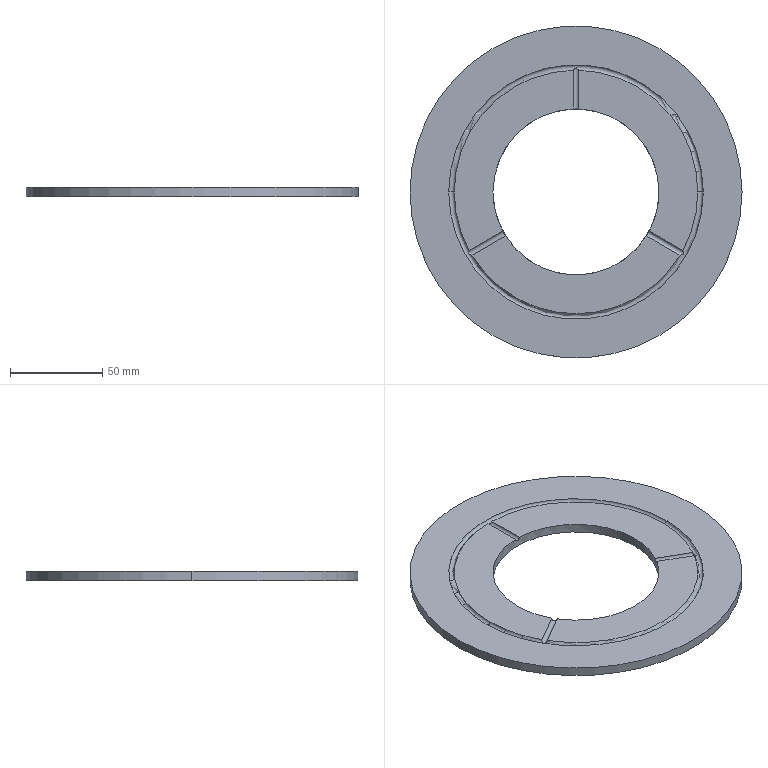Part | SolidWorks | features CirPattern 1, Extrusion 1, ICE 1, SweepCut 1 | 1 solid | 15 faces | box 180 x 180 x 5 mm | volume 93702 mm3 | cylinder 8 | plane 5 | torus 2 | commonest cylinder face diameters 3 x4 90 x2 180 x2
STEP:
#1=CARTESIAN_POINT('',(0.,67.5,3.5));
#2=VERTEX_POINT('',#1);
#3=CARTESIAN_POINT('',(1.5,65.983,5.));
#4=VERTEX_POINT('',#3);
#5=CARTESIAN_POINT('',(0.,67.5,3.5));
#6=CARTESIAN_POINT('',(0.0839,67.416,3.5));
#7=CARTESIAN_POINT('',(0.1692,67.331,3.507));
#8=CARTESIAN_POINT('',(0.3357,67.163,3.536));
#9=CARTESIAN_POINT('',(0.4181,67.081,3.557));
#10=CARTESIAN_POINT('',(0.6621,66.835,3.643));
#11=CARTESIAN_POINT('',(0.8218,66.673,3.731));
#12=CARTESIAN_POINT('',(1.11,66.381,3.974));
#13=CARTESIAN_POINT('',(1.242,66.246,4.131));
#14=CARTESIAN_POINT('',(1.39,66.096,4.425));
#15=CARTESIAN_POINT('',(1.43,66.055,4.531));
#16=CARTESIAN_POINT('',(1.485,65.998,4.758));
#17=CARTESIAN_POINT('',(1.5,65.983,4.879));
#18=CARTESIAN_POINT('',(1.5,65.983,5.));
#19=B_SPLINE_CURVE_WITH_KNOTS('',3,(#5,#6,#7,#8,#9,#10,#11,#12,#13,#14,#15,#16,#17,#18),.UNSPECIFIED.,.F.,.F.,(4,2,2,2,2,2,4),(-0.000007746,0.0003482,0.0007042,0.001416,0.002128,0.002484,0.00284),.UNSPECIFIED.);
#20=EDGE_CURVE('',#2,#4,#19,.T.);
#21=ORIENTED_EDGE('',*,*,#20,.F.);
#22=CARTESIAN_POINT('',(0.,45.,3.5));
#23=VERTEX_POINT('',#22);
#24=CARTESIAN_POINT('',(0.,67.5,3.5));
#25=DIRECTION('',(0.,-1.,0.));
#26=VECTOR('',#25,1000.);
#27=LINE('',#24,#26);
#28=EDGE_CURVE('',#2,#23,#27,.T.);
#29=ORIENTED_EDGE('',*,*,#28,.T.);
#30=CARTESIAN_POINT('',(1.5,44.975,5.));
#31=VERTEX_POINT('',#30);
#32=CARTESIAN_POINT('',(1.5,44.975,5.));
#33=CARTESIAN_POINT('',(1.5,44.975,4.901));
#34=CARTESIAN_POINT('',(1.49,44.975,4.803));
#35=CARTESIAN_POINT('',(1.452,44.977,4.612));
#36=CARTESIAN_POINT('',(1.423,44.978,4.516));
#37=CARTESIAN_POINT('',(1.348,44.98,4.335));
#38=CARTESIAN_POINT('',(1.302,44.981,4.248));
#39=CARTESIAN_POINT('',(1.193,44.984,4.085));
#40=CARTESIAN_POINT('',(1.13,44.986,4.008));
#41=CARTESIAN_POINT('',(0.9218,44.991,3.801));
#42=CARTESIAN_POINT('',(0.7544,44.994,3.689));
#43=CARTESIAN_POINT('',(0.3932,44.999,3.539));
#44=CARTESIAN_POINT('',(0.1957,45.,3.5));
#45=CARTESIAN_POINT('',(0.,45.,3.5));
#46=B_SPLINE_CURVE_WITH_KNOTS('',3,(#32,#33,#34,#35,#36,#37,#38,#39,#40,#41,#42,#43,#44,#45),.UNSPECIFIED.,.F.,.F.,(4,2,2,2,2,2,4),(0.,0.0002932,0.0005864,0.0008796,0.001173,0.001759,0.002346),.UNSPECIFIED.);
#47=EDGE_CURVE('',#31,#23,#46,.T.);
#48=ORIENTED_EDGE('',*,*,#47,.F.);
#49=CARTESIAN_POINT('',(1.5,67.5,5.));
#50=DIRECTION('',(0.,-1.,0.));
#51=VECTOR('',#50,1000.);
#52=LINE('',#49,#51);
#53=EDGE_CURVE('',#4,#31,#52,.T.);
#54=ORIENTED_EDGE('',*,*,#53,.F.);
#55=EDGE_LOOP('',(#21,#29,#48,#54));
#56=FACE_OUTER_BOUND('',#55,.T.);
#57=CARTESIAN_POINT('',(0.,67.5,5.));
#58=DIRECTION('',(0.,-1.,0.));
#59=DIRECTION('',(0.,0.,-1.));
#60=AXIS2_PLACEMENT_3D('',#57,#58,#59);
#61=CYLINDRICAL_SURFACE('',#60,1.5);
#62=ADVANCED_FACE('',(#56),#61,.F.);
#63=CARTESIAN_POINT('',(90.,0.,5.));
#64=VERTEX_POINT('',#63);
#65=CARTESIAN_POINT('',(-90.,0.,5.));
#66=VERTEX_POINT('',#65);
#67=CARTESIAN_POINT('',(0.,0.,5.));
#68=DIRECTION('',(0.,0.,1.));
#69=DIRECTION('',(1.,0.,0.));
#70=AXIS2_PLACEMENT_3D('',#67,#68,#69);
#71=CIRCLE('',#70,90.);
#72=EDGE_CURVE('',#64,#66,#71,.T.);
#73=ORIENTED_EDGE('',*,*,#72,.F.);
#74=CARTESIAN_POINT('',(90.,0.,0.));
#75=VERTEX_POINT('',#74);
#76=CARTESIAN_POINT('',(90.,0.,5.));
#77=DIRECTION('',(0.,0.,-1.));
#78=VECTOR('',#77,1000.);
#79=LINE('',#76,#78);
#80=EDGE_CURVE('',#64,#75,#79,.T.);
#81=ORIENTED_EDGE('',*,*,#80,.T.);
#82=CARTESIAN_POINT('',(-90.,0.,0.));
#83=VERTEX_POINT('',#82);
#84=CARTESIAN_POINT('',(0.,0.,0.));
#85=DIRECTION('',(0.,0.,1.));
#86=DIRECTION('',(1.,0.,0.));
#87=AXIS2_PLACEMENT_3D('',#84,#85,#86);
#88=CIRCLE('',#87,90.);
#89=EDGE_CURVE('',#75,#83,#88,.T.);
#90=ORIENTED_EDGE('',*,*,#89,.T.);
#91=CARTESIAN_POINT('',(-90.,0.,5.));
#92=DIRECTION('',(0.,0.,-1.));
#93=VECTOR('',#92,1000.);
#94=LINE('',#91,#93);
#95=EDGE_CURVE('',#66,#83,#94,.T.);
#96=ORIENTED_EDGE('',*,*,#95,.F.);
#97=EDGE_LOOP('',(#73,#81,#90,#96));
#98=FACE_OUTER_BOUND('',#97,.T.);
#99=CARTESIAN_POINT('',(0.,0.,5.));
#100=DIRECTION('',(0.,0.,-1.));
#101=DIRECTION('',(-1.,0.,0.));
#102=AXIS2_PLACEMENT_3D('',#99,#100,#101);
#103=CYLINDRICAL_SURFACE('',#102,90.);
#104=ADVANCED_FACE('',(#98),#103,.T.);
#105=CARTESIAN_POINT('',(-66.,0.,5.));
#106=VERTEX_POINT('',#105);
#107=CARTESIAN_POINT('',(-57.893,-31.692,5.));
#108=VERTEX_POINT('',#107);
#109=CARTESIAN_POINT('',(0.,0.,5.));
#110=DIRECTION('',(0.,0.,1.));
#111=DIRECTION('',(-1.,0.,0.));
#112=AXIS2_PLACEMENT_3D('',#109,#110,#111);
#113=CIRCLE('',#112,66.);
#114=EDGE_CURVE('',#106,#108,#113,.T.);
#115=ORIENTED_EDGE('',*,*,#114,.F.);
#116=CARTESIAN_POINT('',(-69.,0.,5.));
#117=VERTEX_POINT('',#116);
#118=CARTESIAN_POINT('',(-67.5,0.,5.));
#119=DIRECTION('',(0.,1.,0.));
#120=DIRECTION('',(-1.,0.,0.));
#121=AXIS2_PLACEMENT_3D('',#118,#119,#120);
#122=CIRCLE('',#121,1.5);
#123=EDGE_CURVE('',#106,#117,#122,.T.);
#124=ORIENTED_EDGE('',*,*,#123,.T.);
#125=CARTESIAN_POINT('',(69.,0.,5.));
#126=VERTEX_POINT('',#125);
#127=CARTESIAN_POINT('',(0.,0.,5.));
#128=DIRECTION('',(0.,0.,-1.));
#129=DIRECTION('',(1.,0.,0.));
#130=AXIS2_PLACEMENT_3D('',#127,#128,#129);
#131=CIRCLE('',#130,69.);
#132=EDGE_CURVE('',#126,#117,#131,.T.);
#133=ORIENTED_EDGE('',*,*,#132,.F.);
#134=CARTESIAN_POINT('',(66.,0.,5.));
#135=VERTEX_POINT('',#134);
#136=CARTESIAN_POINT('',(67.5,0.,5.));
#137=DIRECTION('',(0.,-1.,0.));
#138=DIRECTION('',(0.,0.,-1.));
#139=AXIS2_PLACEMENT_3D('',#136,#137,#138);
#140=CIRCLE('',#139,1.5);
#141=EDGE_CURVE('',#135,#126,#140,.T.);
#142=ORIENTED_EDGE('',*,*,#141,.F.);
#143=CARTESIAN_POINT('',(57.893,-31.692,5.));
#144=VERTEX_POINT('',#143);
#145=CARTESIAN_POINT('',(0.,0.,5.));
#146=DIRECTION('',(0.,0.,1.));
#147=DIRECTION('',(-1.,0.,0.));
#148=AXIS2_PLACEMENT_3D('',#145,#146,#147);
#149=CIRCLE('',#148,66.);
#150=EDGE_CURVE('',#144,#135,#149,.T.);
#151=ORIENTED_EDGE('',*,*,#150,.F.);
#152=CARTESIAN_POINT('',(58.457,-33.75,3.5));
#153=VERTEX_POINT('',#152);
#154=CARTESIAN_POINT('',(57.893,-31.692,5.));
#155=CARTESIAN_POINT('',(57.893,-31.692,4.757));
#156=CARTESIAN_POINT('',(57.916,-31.776,4.524));
#157=CARTESIAN_POINT('',(57.992,-32.046,4.133));
#158=CARTESIAN_POINT('',(58.042,-32.226,3.976));
#159=CARTESIAN_POINT('',(58.151,-32.624,3.731));
#160=CARTESIAN_POINT('',(58.21,-32.838,3.645));
#161=CARTESIAN_POINT('',(58.333,-33.289,3.528));
#162=CARTESIAN_POINT('',(58.395,-33.52,3.5));
#163=CARTESIAN_POINT('',(58.457,-33.75,3.5));
#164=B_SPLINE_CURVE_WITH_KNOTS('',3,(#154,#155,#156,#157,#158,#159,#160,#161,#162,#163),.UNSPECIFIED.,.F.,.F.,(4,2,2,2,4),(0.000000196,0.000716,0.001432,0.002147,0.002863),.UNSPECIFIED.);
#165=EDGE_CURVE('',#144,#153,#164,.T.);
#166=ORIENTED_EDGE('',*,*,#165,.T.);
#167=CARTESIAN_POINT('',(56.393,-34.291,5.));
#168=VERTEX_POINT('',#167);
#169=CARTESIAN_POINT('',(58.457,-33.75,3.5));
#170=CARTESIAN_POINT('',(58.342,-33.781,3.5));
#171=CARTESIAN_POINT('',(58.225,-33.812,3.507));
#172=CARTESIAN_POINT('',(57.997,-33.872,3.536));
#173=CARTESIAN_POINT('',(57.885,-33.902,3.557));
#174=CARTESIAN_POINT('',(57.55,-33.991,3.643));
#175=CARTESIAN_POINT('',(57.33,-34.048,3.731));
#176=CARTESIAN_POINT('',(56.932,-34.152,3.974));
#177=CARTESIAN_POINT('',(56.75,-34.199,4.131));
#178=CARTESIAN_POINT('',(56.546,-34.251,4.425));
#179=CARTESIAN_POINT('',(56.49,-34.266,4.531));
#180=CARTESIAN_POINT('',(56.414,-34.285,4.758));
#181=CARTESIAN_POINT('',(56.393,-34.291,4.879));
#182=CARTESIAN_POINT('',(56.393,-34.291,5.));
#183=B_SPLINE_CURVE_WITH_KNOTS('',3,(#169,#170,#171,#172,#173,#174,#175,#176,#177,#178,#179,#180,#181,#182),.UNSPECIFIED.,.F.,.F.,(4,2,2,2,2,2,4),(-0.000007746,0.0003482,0.0007042,0.001416,0.002128,0.002484,0.00284),.UNSPECIFIED.);
#184=EDGE_CURVE('',#153,#168,#183,.T.);
#185=ORIENTED_EDGE('',*,*,#184,.T.);
#186=CARTESIAN_POINT('',(-56.393,-34.291,5.));
#187=VERTEX_POINT('',#186);
#188=CARTESIAN_POINT('',(0.,0.,5.));
#189=DIRECTION('',(0.,0.,1.));
#190=DIRECTION('',(-1.,0.,0.));
#191=AXIS2_PLACEMENT_3D('',#188,#189,#190);
#192=CIRCLE('',#191,66.);
#193=EDGE_CURVE('',#187,#168,#192,.T.);
#194=ORIENTED_EDGE('',*,*,#193,.F.);
#195=CARTESIAN_POINT('',(-58.457,-33.75,3.5));
#196=VERTEX_POINT('',#195);
#197=CARTESIAN_POINT('',(-56.393,-34.291,5.));
#198=CARTESIAN_POINT('',(-56.393,-34.291,4.757));
#199=CARTESIAN_POINT('',(-56.477,-34.269,4.524));
#200=CARTESIAN_POINT('',(-56.748,-34.199,4.133));
#201=CARTESIAN_POINT('',(-56.929,-34.153,3.976));
#202=CARTESIAN_POINT('',(-57.329,-34.049,3.731));
#203=CARTESIAN_POINT('',(-57.544,-33.992,3.645));
#204=CARTESIAN_POINT('',(-57.995,-33.873,3.528));
#205=CARTESIAN_POINT('',(-58.226,-33.812,3.5));
#206=CARTESIAN_POINT('',(-58.457,-33.75,3.5));
#207=B_SPLINE_CURVE_WITH_KNOTS('',3,(#197,#198,#199,#200,#201,#202,#203,#204,#205,#206),.UNSPECIFIED.,.F.,.F.,(4,2,2,2,4),(0.000000196,0.000716,0.001432,0.002147,0.002863),.UNSPECIFIED.);
#208=EDGE_CURVE('',#187,#196,#207,.T.);
#209=ORIENTED_EDGE('',*,*,#208,.T.);
#210=CARTESIAN_POINT('',(-58.457,-33.75,3.5));
#211=CARTESIAN_POINT('',(-58.426,-33.635,3.5));
#212=CARTESIAN_POINT('',(-58.395,-33.519,3.507));
#213=CARTESIAN_POINT('',(-58.333,-33.291,3.536));
#214=CARTESIAN_POINT('',(-58.303,-33.178,3.557));
#215=CARTESIAN_POINT('',(-58.212,-32.844,3.643));
#216=CARTESIAN_POINT('',(-58.152,-32.625,3.731));
#217=CARTESIAN_POINT('',(-58.042,-32.229,3.974));
#218=CARTESIAN_POINT('',(-57.992,-32.048,4.131));
#219=CARTESIAN_POINT('',(-57.935,-31.844,4.425));
#220=CARTESIAN_POINT('',(-57.92,-31.789,4.531));
#221=CARTESIAN_POINT('',(-57.899,-31.713,4.758));
#222=CARTESIAN_POINT('',(-57.893,-31.692,4.879));
#223=CARTESIAN_POINT('',(-57.893,-31.692,5.));
#224=B_SPLINE_CURVE_WITH_KNOTS('',3,(#210,#211,#212,#213,#214,#215,#216,#217,#218,#219,#220,#221,#222,#223),.UNSPECIFIED.,.F.,.F.,(4,2,2,2,2,2,4),(-0.000007746,0.0003482,0.0007042,0.001416,0.002128,0.002484,0.00284),.UNSPECIFIED.);
#225=EDGE_CURVE('',#196,#108,#224,.T.);
#226=ORIENTED_EDGE('',*,*,#225,.T.);
#227=EDGE_LOOP('',(#115,#124,#133,#142,#151,#166,#185,#194,#209,#226));
#228=FACE_OUTER_BOUND('',#227,.T.);
#229=CARTESIAN_POINT('',(0.,0.,5.));
#230=DIRECTION('',(0.,0.,1.));
#231=DIRECTION('',(1.,0.,0.));
#232=AXIS2_PLACEMENT_3D('',#229,#230,#231);
#233=TOROIDAL_SURFACE('',#232,67.5,1.5);
#234=ADVANCED_FACE('',(#228),#233,.F.);
#235=CARTESIAN_POINT('',(39.699,-21.188,5.));
#236=VERTEX_POINT('',#235);
#237=CARTESIAN_POINT('',(45.,0.,5.));
#238=VERTEX_POINT('',#237);
#239=CARTESIAN_POINT('',(0.,0.,5.));
#240=DIRECTION('',(0.,0.,1.));
#241=DIRECTION('',(1.,0.,0.));
#242=AXIS2_PLACEMENT_3D('',#239,#240,#241);
#243=CIRCLE('',#242,45.);
#244=EDGE_CURVE('',#236,#238,#243,.T.);
#245=ORIENTED_EDGE('',*,*,#244,.T.);
#246=CARTESIAN_POINT('',(45.,0.,0.));
#247=VERTEX_POINT('',#246);
#248=CARTESIAN_POINT('',(45.,0.,5.));
#249=DIRECTION('',(0.,0.,-1.));
#250=VECTOR('',#249,1000.);
#251=LINE('',#248,#250);
#252=EDGE_CURVE('',#238,#247,#251,.T.);
#253=ORIENTED_EDGE('',*,*,#252,.T.);
#254=CARTESIAN_POINT('',(-45.,0.,0.));
#255=VERTEX_POINT('',#254);
#256=CARTESIAN_POINT('',(0.,0.,0.));
#257=DIRECTION('',(0.,0.,1.));
#258=DIRECTION('',(1.,0.,0.));
#259=AXIS2_PLACEMENT_3D('',#256,#257,#258);
#260=CIRCLE('',#259,45.);
#261=EDGE_CURVE('',#255,#247,#260,.T.);
#262=ORIENTED_EDGE('',*,*,#261,.F.);
#263=CARTESIAN_POINT('',(-45.,0.,5.));
#264=VERTEX_POINT('',#263);
#265=CARTESIAN_POINT('',(-45.,0.,5.));
#266=DIRECTION('',(0.,0.,-1.));
#267=VECTOR('',#266,1000.);
#268=LINE('',#265,#267);
#269=EDGE_CURVE('',#264,#255,#268,.T.);
#270=ORIENTED_EDGE('',*,*,#269,.F.);
#271=CARTESIAN_POINT('',(-39.699,-21.188,5.));
#272=VERTEX_POINT('',#271);
#273=CARTESIAN_POINT('',(0.,0.,5.));
#274=DIRECTION('',(0.,0.,1.));
#275=DIRECTION('',(1.,0.,0.));
#276=AXIS2_PLACEMENT_3D('',#273,#274,#275);
#277=CIRCLE('',#276,45.);
#278=EDGE_CURVE('',#264,#272,#277,.T.);
#279=ORIENTED_EDGE('',*,*,#278,.T.);
#280=CARTESIAN_POINT('',(-38.199,-23.787,5.));
#281=VERTEX_POINT('',#280);
#282=CARTESIAN_POINT('',(-39.699,-21.188,5.));
#283=CARTESIAN_POINT('',(-39.699,-21.188,4.901));
#284=CARTESIAN_POINT('',(-39.695,-21.197,4.803));
#285=CARTESIAN_POINT('',(-39.677,-21.231,4.612));
#286=CARTESIAN_POINT('',(-39.663,-21.256,4.516));
#287=CARTESIAN_POINT('',(-39.628,-21.323,4.335));
#288=CARTESIAN_POINT('',(-39.606,-21.363,4.249));
#289=CARTESIAN_POINT('',(-39.554,-21.459,4.086));
#290=CARTESIAN_POINT('',(-39.524,-21.515,4.008));
#291=CARTESIAN_POINT('',(-39.424,-21.697,3.801));
#292=CARTESIAN_POINT('',(-39.343,-21.843,3.689));
#293=CARTESIAN_POINT('',(-39.167,-22.158,3.539));
#294=CARTESIAN_POINT('',(-39.069,-22.33,3.5));
#295=CARTESIAN_POINT('',(-38.922,-22.584,3.5));
#296=CARTESIAN_POINT('',(-38.873,-22.67,3.51));
#297=CARTESIAN_POINT('',(-38.775,-22.836,3.548));
#298=CARTESIAN_POINT('',(-38.728,-22.917,3.576));
#299=CARTESIAN_POINT('',(-38.635,-23.073,3.651));
#300=CARTESIAN_POINT('',(-38.59,-23.148,3.698));
#301=CARTESIAN_POINT('',(-38.506,-23.287,3.807));
#302=CARTESIAN_POINT('',(-38.467,-23.352,3.869));
#303=CARTESIAN_POINT('',(-38.357,-23.532,4.079));
#304=CARTESIAN_POINT('',(-38.299,-23.625,4.244));
#305=CARTESIAN_POINT('',(-38.24,-23.722,4.517));
#306=CARTESIAN_POINT('',(-38.225,-23.746,4.61));
#307=CARTESIAN_POINT('',(-38.205,-23.778,4.803));
#308=CARTESIAN_POINT('',(-38.199,-23.787,4.902));
#309=CARTESIAN_POINT('',(-38.199,-23.787,5.));
#310=B_SPLINE_CURVE_WITH_KNOTS('',3,(#282,#283,#284,#285,#286,#287,#288,#289,#290,#291,#292,#293,#294,#295,#296,#297,#298,#299,#300,#301,#302,#303,#304,#305,#306,#307,#308,#309),.UNSPECIFIED.,.F.,.F.,(4,2,2,2,2,2,2,2,2,2,2,2,2,4),(0.,0.0002931,0.0005863,0.0008794,0.001173,0.001759,0.002345,0.002638,0.002931,0.003224,0.003518,0.004104,0.004397,0.00469),.UNSPECIFIED.);
#311=EDGE_CURVE('',#272,#281,#310,.T.);
#312=ORIENTED_EDGE('',*,*,#311,.T.);
#313=CARTESIAN_POINT('',(38.199,-23.787,5.));
#314=VERTEX_POINT('',#313);
#315=CARTESIAN_POINT('',(0.,0.,5.));
#316=DIRECTION('',(0.,0.,1.));
#317=DIRECTION('',(1.,0.,0.));
#318=AXIS2_PLACEMENT_3D('',#315,#316,#317);
#319=CIRCLE('',#318,45.);
#320=EDGE_CURVE('',#281,#314,#319,.T.);
#321=ORIENTED_EDGE('',*,*,#320,.T.);
#322=CARTESIAN_POINT('',(38.199,-23.787,5.));
#323=CARTESIAN_POINT('',(38.199,-23.787,4.901));
#324=CARTESIAN_POINT('',(38.205,-23.778,4.803));
#325=CARTESIAN_POINT('',(38.225,-23.746,4.612));
#326=CARTESIAN_POINT('',(38.24,-23.721,4.516));
#327=CARTESIAN_POINT('',(38.28,-23.657,4.335));
#328=CARTESIAN_POINT('',(38.304,-23.618,4.249));
#329=CARTESIAN_POINT('',(38.361,-23.525,4.086));
#330=CARTESIAN_POINT('',(38.394,-23.471,4.008));
#331=CARTESIAN_POINT('',(38.502,-23.294,3.801));
#332=CARTESIAN_POINT('',(38.589,-23.151,3.689));
#333=CARTESIAN_POINT('',(38.773,-22.84,3.539));
#334=CARTESIAN_POINT('',(38.873,-22.67,3.5));
#335=CARTESIAN_POINT('',(39.02,-22.416,3.5));
#336=CARTESIAN_POINT('',(39.069,-22.329,3.51));
#337=CARTESIAN_POINT('',(39.164,-22.162,3.548));
#338=CARTESIAN_POINT('',(39.21,-22.081,3.576));
#339=CARTESIAN_POINT('',(39.299,-21.922,3.651));
#340=CARTESIAN_POINT('',(39.342,-21.846,3.698));
#341=CARTESIAN_POINT('',(39.42,-21.703,3.807));
#342=CARTESIAN_POINT('',(39.457,-21.637,3.869));
#343=CARTESIAN_POINT('',(39.558,-21.452,4.079));
#344=CARTESIAN_POINT('',(39.61,-21.356,4.244));
#345=CARTESIAN_POINT('',(39.663,-21.256,4.517));
#346=CARTESIAN_POINT('',(39.677,-21.231,4.61));
#347=CARTESIAN_POINT('',(39.695,-21.197,4.803));
#348=CARTESIAN_POINT('',(39.699,-21.188,4.902));
#349=CARTESIAN_POINT('',(39.699,-21.188,5.));
#350=B_SPLINE_CURVE_WITH_KNOTS('',3,(#322,#323,#324,#325,#326,#327,#328,#329,#330,#331,#332,#333,#334,#335,#336,#337,#338,#339,#340,#341,#342,#343,#344,#345,#346,#347,#348,#349),.UNSPECIFIED.,.F.,.F.,(4,2,2,2,2,2,2,2,2,2,2,2,2,4),(0.,0.0002931,0.0005863,0.0008794,0.001173,0.001759,0.002345,0.002638,0.002931,0.003224,0.003518,0.004104,0.004397,0.00469),.UNSPECIFIED.);
#351=EDGE_CURVE('',#314,#236,#350,.T.);
#352=ORIENTED_EDGE('',*,*,#351,.T.);
#353=EDGE_LOOP('',(#245,#253,#262,#270,#279,#312,#321,#352));
#354=FACE_OUTER_BOUND('',#353,.T.);
#355=CARTESIAN_POINT('',(0.,0.,5.));
#356=DIRECTION('',(0.,0.,-1.));
#357=DIRECTION('',(-1.,0.,0.));
#358=AXIS2_PLACEMENT_3D('',#355,#356,#357);
#359=CYLINDRICAL_SURFACE('',#358,45.);
#360=ADVANCED_FACE('',(#354),#359,.F.);
#361=ORIENTED_EDGE('',*,*,#244,.F.);
#362=CARTESIAN_POINT('',(59.207,-32.451,5.));
#363=DIRECTION('',(0.866,-0.5,0.));
#364=VECTOR('',#363,1000.);
#365=LINE('',#362,#364);
#366=EDGE_CURVE('',#236,#144,#365,.T.);
#367=ORIENTED_EDGE('',*,*,#366,.T.);
#368=ORIENTED_EDGE('',*,*,#150,.T.);
#369=CARTESIAN_POINT('',(0.,0.,5.));
#370=DIRECTION('',(0.,0.,1.));
#371=DIRECTION('',(-1.,0.,0.));
#372=AXIS2_PLACEMENT_3D('',#369,#370,#371);
#373=CIRCLE('',#372,66.);
#374=EDGE_CURVE('',#135,#4,#373,.T.);
#375=ORIENTED_EDGE('',*,*,#374,.T.);
#376=ORIENTED_EDGE('',*,*,#53,.T.);
#377=CARTESIAN_POINT('',(0.,0.,5.));
#378=DIRECTION('',(0.,0.,1.));
#379=DIRECTION('',(1.,0.,0.));
#380=AXIS2_PLACEMENT_3D('',#377,#378,#379);
#381=CIRCLE('',#380,45.);
#382=EDGE_CURVE('',#238,#31,#381,.T.);
#383=ORIENTED_EDGE('',*,*,#382,.F.);
#384=EDGE_LOOP('',(#361,#367,#368,#375,#376,#383));
#385=FACE_OUTER_BOUND('',#384,.T.);
#386=CARTESIAN_POINT('',(0.,0.,5.));
#387=DIRECTION('',(0.,0.,1.));
#388=DIRECTION('',(1.,0.,0.));
#389=AXIS2_PLACEMENT_3D('',#386,#387,#388);
#390=PLANE('',#389);
#391=ADVANCED_FACE('',(#385),#390,.T.);
#392=ORIENTED_EDGE('',*,*,#193,.T.);
#393=CARTESIAN_POINT('',(57.707,-35.049,5.));
#394=DIRECTION('',(-0.866,0.5,0.));
#395=VECTOR('',#394,1000.);
#396=LINE('',#393,#395);
#397=EDGE_CURVE('',#168,#314,#396,.T.);
#398=ORIENTED_EDGE('',*,*,#397,.T.);
#399=ORIENTED_EDGE('',*,*,#320,.F.);
#400=CARTESIAN_POINT('',(-57.707,-35.049,5.));
#401=DIRECTION('',(-0.866,-0.5,0.));
#402=VECTOR('',#401,1000.);
#403=LINE('',#400,#402);
#404=EDGE_CURVE('',#281,#187,#403,.T.);
#405=ORIENTED_EDGE('',*,*,#404,.T.);
#406=EDGE_LOOP('',(#392,#398,#399,#405));
#407=FACE_OUTER_BOUND('',#406,.T.);
#408=CARTESIAN_POINT('',(0.,0.,5.));
#409=DIRECTION('',(0.,0.,1.));
#410=DIRECTION('',(1.,0.,0.));
#411=AXIS2_PLACEMENT_3D('',#408,#409,#410);
#412=PLANE('',#411);
#413=ADVANCED_FACE('',(#407),#412,.T.);
#414=CARTESIAN_POINT('',(-1.5,65.983,5.));
#415=VERTEX_POINT('',#414);
#416=CARTESIAN_POINT('',(0.,0.,5.));
#417=DIRECTION('',(0.,0.,1.));
#418=DIRECTION('',(-1.,0.,0.));
#419=AXIS2_PLACEMENT_3D('',#416,#417,#418);
#420=CIRCLE('',#419,66.);
#421=EDGE_CURVE('',#415,#106,#420,.T.);
#422=ORIENTED_EDGE('',*,*,#421,.T.);
#423=ORIENTED_EDGE('',*,*,#114,.T.);
#424=CARTESIAN_POINT('',(-59.207,-32.451,5.));
#425=DIRECTION('',(0.866,0.5,0.));
#426=VECTOR('',#425,1000.);
#427=LINE('',#424,#426);
#428=EDGE_CURVE('',#108,#272,#427,.T.);
#429=ORIENTED_EDGE('',*,*,#428,.T.);
#430=ORIENTED_EDGE('',*,*,#278,.F.);
#431=CARTESIAN_POINT('',(-1.5,44.975,5.));
#432=VERTEX_POINT('',#431);
#433=CARTESIAN_POINT('',(0.,0.,5.));
#434=DIRECTION('',(0.,0.,1.));
#435=DIRECTION('',(1.,0.,0.));
#436=AXIS2_PLACEMENT_3D('',#433,#434,#435);
#437=CIRCLE('',#436,45.);
#438=EDGE_CURVE('',#432,#264,#437,.T.);
#439=ORIENTED_EDGE('',*,*,#438,.F.);
#440=CARTESIAN_POINT('',(-1.5,67.5,5.));
#441=DIRECTION('',(0.,1.,0.));
#442=VECTOR('',#441,1000.);
#443=LINE('',#440,#442);
#444=EDGE_CURVE('',#432,#415,#443,.T.);
#445=ORIENTED_EDGE('',*,*,#444,.T.);
#446=EDGE_LOOP('',(#422,#423,#429,#430,#439,#445));
#447=FACE_OUTER_BOUND('',#446,.T.);
#448=CARTESIAN_POINT('',(0.,0.,5.));
#449=DIRECTION('',(0.,0.,1.));
#450=DIRECTION('',(1.,0.,0.));
#451=AXIS2_PLACEMENT_3D('',#448,#449,#450);
#452=PLANE('',#451);
#453=ADVANCED_FACE('',(#447),#452,.T.);
#454=ORIENTED_EDGE('',*,*,#252,.F.);
#455=ORIENTED_EDGE('',*,*,#382,.T.);
#456=ORIENTED_EDGE('',*,*,#47,.T.);
#457=CARTESIAN_POINT('',(0.,45.,3.5));
#458=CARTESIAN_POINT('',(-0.09778,45.,3.5));
#459=CARTESIAN_POINT('',(-0.1971,45.,3.51));
#460=CARTESIAN_POINT('',(-0.3894,44.998,3.548));
#461=CARTESIAN_POINT('',(-0.4828,44.998,3.576));
#462=CARTESIAN_POINT('',(-0.6643,44.995,3.652));
#463=CARTESIAN_POINT('',(-0.7521,44.994,3.698));
#464=CARTESIAN_POINT('',(-0.9145,44.991,3.807));
#465=CARTESIAN_POINT('',(-0.9903,44.989,3.869));
#466=CARTESIAN_POINT('',(-1.2,44.984,4.079));
#467=CARTESIAN_POINT('',(-1.31,44.981,4.244));
#468=CARTESIAN_POINT('',(-1.461,44.976,4.607));
#469=CARTESIAN_POINT('',(-1.5,44.975,4.802));
#470=CARTESIAN_POINT('',(-1.5,44.975,5.));
#471=B_SPLINE_CURVE_WITH_KNOTS('',3,(#457,#458,#459,#460,#461,#462,#463,#464,#465,#466,#467,#468,#469,#470),.UNSPECIFIED.,.F.,.F.,(4,2,2,2,2,2,4),(0.002346,0.002638,0.002931,0.003224,0.003517,0.004103,0.004689),.UNSPECIFIED.);
#472=EDGE_CURVE('',#23,#432,#471,.T.);
#473=ORIENTED_EDGE('',*,*,#472,.T.);
#474=ORIENTED_EDGE('',*,*,#438,.T.);
#475=ORIENTED_EDGE('',*,*,#269,.T.);
#476=CARTESIAN_POINT('',(0.,0.,0.));
#477=DIRECTION('',(0.,0.,1.));
#478=DIRECTION('',(1.,0.,0.));
#479=AXIS2_PLACEMENT_3D('',#476,#477,#478);
#480=CIRCLE('',#479,45.);
#481=EDGE_CURVE('',#247,#255,#480,.T.);
#482=ORIENTED_EDGE('',*,*,#481,.F.);
#483=EDGE_LOOP('',(#454,#455,#456,#473,#474,#475,#482));
#484=FACE_OUTER_BOUND('',#483,.T.);
#485=CARTESIAN_POINT('',(0.,0.,5.));
#486=DIRECTION('',(0.,0.,-1.));
#487=DIRECTION('',(-1.,0.,0.));
#488=AXIS2_PLACEMENT_3D('',#485,#486,#487);
#489=CYLINDRICAL_SURFACE('',#488,45.);
#490=ADVANCED_FACE('',(#484),#489,.F.);
#491=ORIENTED_EDGE('',*,*,#123,.F.);
#492=ORIENTED_EDGE('',*,*,#421,.F.);
#493=CARTESIAN_POINT('',(-1.5,65.983,5.));
#494=CARTESIAN_POINT('',(-1.5,65.983,4.757));
#495=CARTESIAN_POINT('',(-1.439,66.045,4.524));
#496=CARTESIAN_POINT('',(-1.243,66.245,4.133));
#497=CARTESIAN_POINT('',(-1.112,66.379,3.976));
#498=CARTESIAN_POINT('',(-0.8224,66.673,3.731));
#499=CARTESIAN_POINT('',(-0.6665,66.83,3.645));
#500=CARTESIAN_POINT('',(-0.3376,67.162,3.528));
#501=CARTESIAN_POINT('',(-0.1687,67.331,3.5));
#502=CARTESIAN_POINT('',(0.,67.5,3.5));
#503=B_SPLINE_CURVE_WITH_KNOTS('',3,(#493,#494,#495,#496,#497,#498,#499,#500,#501,#502),.UNSPECIFIED.,.F.,.F.,(4,2,2,2,4),(0.000000196,0.000716,0.001432,0.002147,0.002863),.UNSPECIFIED.);
#504=EDGE_CURVE('',#415,#2,#503,.T.);
#505=ORIENTED_EDGE('',*,*,#504,.T.);
#506=ORIENTED_EDGE('',*,*,#20,.T.);
#507=ORIENTED_EDGE('',*,*,#374,.F.);
#508=ORIENTED_EDGE('',*,*,#141,.T.);
#509=CARTESIAN_POINT('',(0.,0.,5.));
#510=DIRECTION('',(0.,0.,-1.));
#511=DIRECTION('',(1.,0.,0.));
#512=AXIS2_PLACEMENT_3D('',#509,#510,#511);
#513=CIRCLE('',#512,69.);
#514=EDGE_CURVE('',#117,#126,#513,.T.);
#515=ORIENTED_EDGE('',*,*,#514,.F.);
#516=EDGE_LOOP('',(#491,#492,#505,#506,#507,#508,#515));
#517=FACE_OUTER_BOUND('',#516,.T.);
#518=CARTESIAN_POINT('',(0.,0.,5.));
#519=DIRECTION('',(0.,0.,1.));
#520=DIRECTION('',(1.,0.,0.));
#521=AXIS2_PLACEMENT_3D('',#518,#519,#520);
#522=TOROIDAL_SURFACE('',#521,67.5,1.5);
#523=ADVANCED_FACE('',(#517),#522,.F.);
#524=CARTESIAN_POINT('',(0.,0.,5.));
#525=DIRECTION('',(0.,0.,1.));
#526=DIRECTION('',(1.,0.,0.));
#527=AXIS2_PLACEMENT_3D('',#524,#525,#526);
#528=CIRCLE('',#527,90.);
#529=EDGE_CURVE('',#66,#64,#528,.T.);
#530=ORIENTED_EDGE('',*,*,#529,.T.);
#531=ORIENTED_EDGE('',*,*,#72,.T.);
#532=EDGE_LOOP('',(#530,#531));
#533=FACE_OUTER_BOUND('',#532,.T.);
#534=ORIENTED_EDGE('',*,*,#132,.T.);
#535=ORIENTED_EDGE('',*,*,#514,.T.);
#536=EDGE_LOOP('',(#534,#535));
#537=FACE_BOUND('',#536,.T.);
#538=CARTESIAN_POINT('',(0.,0.,5.));
#539=DIRECTION('',(0.,0.,1.));
#540=DIRECTION('',(1.,0.,0.));
#541=AXIS2_PLACEMENT_3D('',#538,#539,#540);
#542=PLANE('',#541);
#543=ADVANCED_FACE('',(#533,#537),#542,.T.);
#544=CARTESIAN_POINT('',(0.,0.,0.));
#545=DIRECTION('',(0.,0.,1.));
#546=DIRECTION('',(1.,0.,0.));
#547=AXIS2_PLACEMENT_3D('',#544,#545,#546);
#548=CIRCLE('',#547,90.);
#549=EDGE_CURVE('',#83,#75,#548,.T.);
#550=ORIENTED_EDGE('',*,*,#549,.F.);
#551=ORIENTED_EDGE('',*,*,#89,.F.);
#552=EDGE_LOOP('',(#550,#551));
#553=FACE_OUTER_BOUND('',#552,.T.);
#554=ORIENTED_EDGE('',*,*,#261,.T.);
#555=ORIENTED_EDGE('',*,*,#481,.T.);
#556=EDGE_LOOP('',(#554,#555));
#557=FACE_BOUND('',#556,.T.);
#558=CARTESIAN_POINT('',(0.,0.,0.));
#559=DIRECTION('',(0.,0.,1.));
#560=DIRECTION('',(1.,0.,0.));
#561=AXIS2_PLACEMENT_3D('',#558,#559,#560);
#562=PLANE('',#561);
#563=ADVANCED_FACE('',(#553,#557),#562,.F.);
#564=ORIENTED_EDGE('',*,*,#80,.F.);
#565=ORIENTED_EDGE('',*,*,#529,.F.);
#566=ORIENTED_EDGE('',*,*,#95,.T.);
#567=ORIENTED_EDGE('',*,*,#549,.T.);
#568=EDGE_LOOP('',(#564,#565,#566,#567));
#569=FACE_OUTER_BOUND('',#568,.T.);
#570=CARTESIAN_POINT('',(0.,0.,5.));
#571=DIRECTION('',(0.,0.,-1.));
#572=DIRECTION('',(-1.,0.,0.));
#573=AXIS2_PLACEMENT_3D('',#570,#571,#572);
#574=CYLINDRICAL_SURFACE('',#573,90.);
#575=ADVANCED_FACE('',(#569),#574,.T.);
#576=ORIENTED_EDGE('',*,*,#28,.F.);
#577=ORIENTED_EDGE('',*,*,#504,.F.);
#578=ORIENTED_EDGE('',*,*,#444,.F.);
#579=ORIENTED_EDGE('',*,*,#472,.F.);
#580=EDGE_LOOP('',(#576,#577,#578,#579));
#581=FACE_OUTER_BOUND('',#580,.T.);
#582=CARTESIAN_POINT('',(0.,67.5,5.));
#583=DIRECTION('',(0.,-1.,0.));
#584=DIRECTION('',(0.,0.,-1.));
#585=AXIS2_PLACEMENT_3D('',#582,#583,#584);
#586=CYLINDRICAL_SURFACE('',#585,1.5);
#587=ADVANCED_FACE('',(#581),#586,.F.);
#588=ORIENTED_EDGE('',*,*,#428,.F.);
#589=ORIENTED_EDGE('',*,*,#225,.F.);
#590=ORIENTED_EDGE('',*,*,#208,.F.);
#591=ORIENTED_EDGE('',*,*,#404,.F.);
#592=ORIENTED_EDGE('',*,*,#311,.F.);
#593=EDGE_LOOP('',(#588,#589,#590,#591,#592));
#594=FACE_OUTER_BOUND('',#593,.T.);
#595=CARTESIAN_POINT('',(-58.457,-33.75,5.));
#596=DIRECTION('',(0.866,0.5,0.));
#597=DIRECTION('',(-0.5,0.866,0.));
#598=AXIS2_PLACEMENT_3D('',#595,#596,#597);
#599=CYLINDRICAL_SURFACE('',#598,1.5);
#600=ADVANCED_FACE('',(#594),#599,.F.);
#601=ORIENTED_EDGE('',*,*,#397,.F.);
#602=ORIENTED_EDGE('',*,*,#184,.F.);
#603=ORIENTED_EDGE('',*,*,#165,.F.);
#604=ORIENTED_EDGE('',*,*,#366,.F.);
#605=ORIENTED_EDGE('',*,*,#351,.F.);
#606=EDGE_LOOP('',(#601,#602,#603,#604,#605));
#607=FACE_OUTER_BOUND('',#606,.T.);
#608=CARTESIAN_POINT('',(58.457,-33.75,5.));
#609=DIRECTION('',(-0.866,0.5,0.));
#610=DIRECTION('',(-0.5,-0.866,0.));
#611=AXIS2_PLACEMENT_3D('',#608,#609,#610);
#612=CYLINDRICAL_SURFACE('',#611,1.5);
#613=ADVANCED_FACE('',(#607),#612,.F.);
#614=CLOSED_SHELL('',(#62,#104,#234,#360,#391,#413,#453,#490,#523,#543,#563,#575,#587,#600,#613));
#615=MANIFOLD_SOLID_BREP('',#614);
#616=CARTESIAN_POINT('',(0.,0.,0.));
#617=DIRECTION('',(0.,0.,1.));
#618=DIRECTION('',(1.,0.,0.));
#619=AXIS2_PLACEMENT_3D('',#616,#617,#618);
#620=(LENGTH_UNIT()NAMED_UNIT(*)SI_UNIT(.MILLI.,.METRE.));
#621=UNCERTAINTY_MEASURE_WITH_UNIT(LENGTH_MEASURE(0.00001),#620,'','');
#622=(NAMED_UNIT(*)PLANE_ANGLE_UNIT()SI_UNIT($,.RADIAN.));
#623=(NAMED_UNIT(*)SI_UNIT($,.STERADIAN.)SOLID_ANGLE_UNIT());
#624=(GEOMETRIC_REPRESENTATION_CONTEXT(3)GLOBAL_UNCERTAINTY_ASSIGNED_CONTEXT((#621))GLOBAL_UNIT_ASSIGNED_CONTEXT((#620,#622,#623))REPRESENTATION_CONTEXT('',''));
#625=ADVANCED_BREP_SHAPE_REPRESENTATION('',(#615,#619),#624);